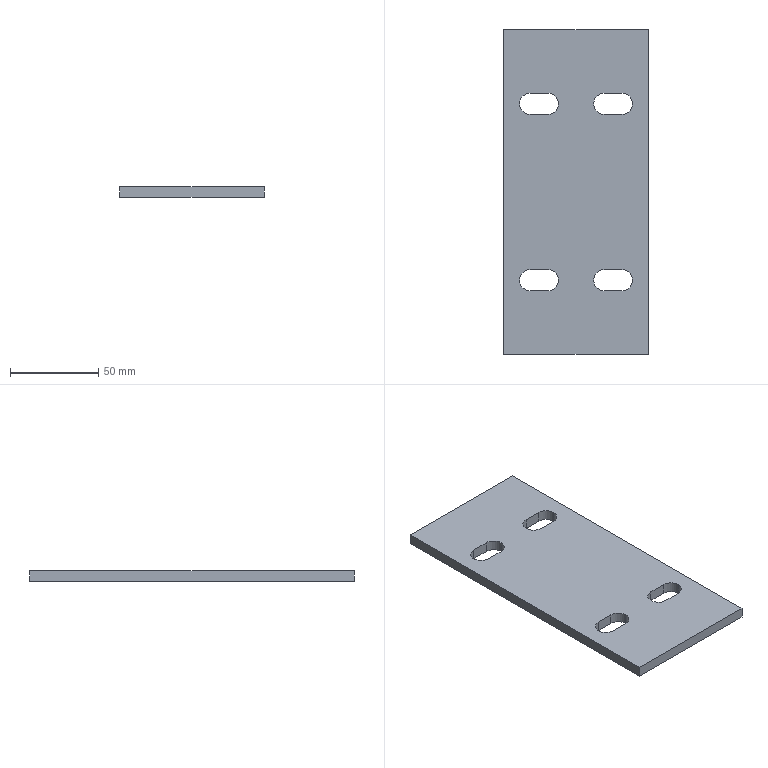Part | STEP file | 护栏连接Plate 200-2 | 1 solid | 26 faces | box 82 x 184 x 6 mm | volume 84934 mm3 | plane 14 | cylinder 12 | commonest cylinder face diameters 12 x12